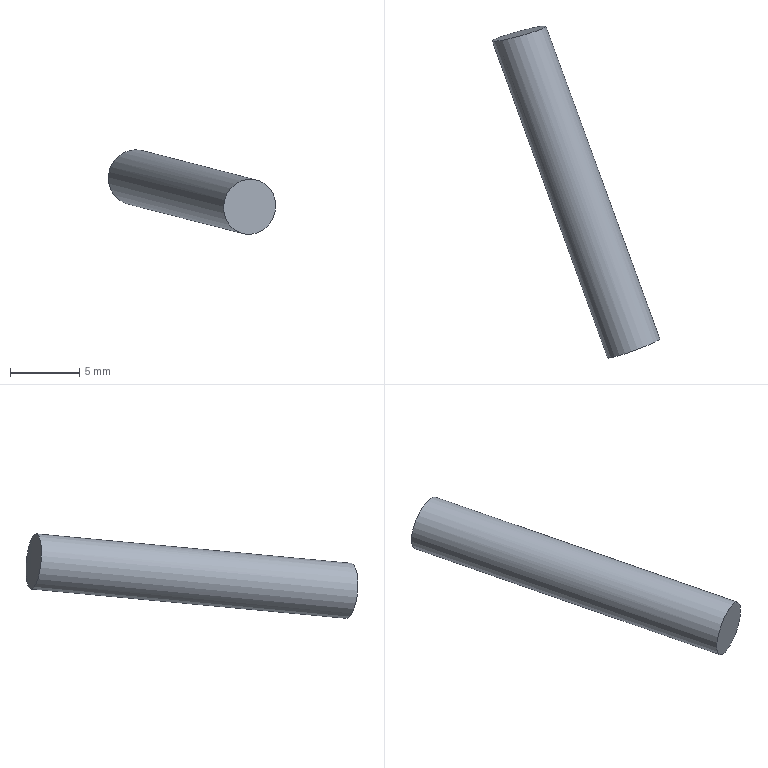Part | NX | features solid 2 | 1 solid | 3 faces | box 12.083 x 23.968 x 6.098 mm | volume 304.751 mm3 | cylinder 1 | plane 1 | spline 1 | commonest cylinder face diameters 4 x1
STEP:
#1=CARTESIAN_POINT('',(652.376,51.525,-28.692));
#2=VERTEX_POINT('',#1);
#3=CARTESIAN_POINT('',(652.847,51.506,-27.131));
#4=CARTESIAN_POINT('',(652.164,51.468,-28.691));
#5=CARTESIAN_POINT('',(652.75,51.771,-30.259));
#6=CARTESIAN_POINT('',(654.244,52.235,-30.913));
#7=CARTESIAN_POINT('',(655.778,52.598,-30.282));
#8=CARTESIAN_POINT('',(656.457,52.642,-28.723));
#9=CARTESIAN_POINT('',(655.876,52.335,-27.157));
#10=CARTESIAN_POINT('',(654.383,51.863,-26.501));
#11=CARTESIAN_POINT('',(652.847,51.506,-27.131));
#12=CARTESIAN_POINT('',(652.164,51.468,-28.691));
#13=CARTESIAN_POINT('',(652.75,51.771,-30.259));
#14=B_SPLINE_CURVE_WITH_KNOTS('',3,(#3,#4,#5,#6,#7,#8,#9,#10,#11,#12,#13),.UNSPECIFIED.,.T.,.F.,(1,1,1,1,1,1,1,1,1,1,1,1,1,1,1),(-0.004697,-0.003132,-0.001566,0.,0.001566,0.003132,0.004697,0.006263,0.007829,0.009395,0.01096,0.01253,0.01409,0.01566,0.01722),.UNSPECIFIED.);
#15=EDGE_CURVE('',#2,#2,#14,.T.);
#16=ORIENTED_EDGE('',*,*,#15,.T.);
#17=EDGE_LOOP('',(#16));
#18=FACE_BOUND('',#17,.T.);
#19=CARTESIAN_POINT('',(660.698,28.66,-30.821));
#20=VERTEX_POINT('',#19);
#21=CARTESIAN_POINT('',(662.577,29.344,-30.821));
#22=DIRECTION('',(-0.3407,0.9361,0.08716));
#23=DIRECTION('',(-0.9397,-0.342,0.));
#24=AXIS2_PLACEMENT_3D('',#21,#22,#23);
#25=CIRCLE('',#24,2.);
#26=EDGE_CURVE('',#20,#20,#25,.T.);
#27=ORIENTED_EDGE('',*,*,#26,.T.);
#28=EDGE_LOOP('',(#27));
#29=FACE_BOUND('',#28,.T.);
#30=CARTESIAN_POINT('',(654.059,52.747,-28.642));
#31=DIRECTION('',(0.3407,-0.9361,-0.08716));
#32=DIRECTION('',(-0.9397,-0.342,0.));
#33=AXIS2_PLACEMENT_3D('',#30,#31,#32);
#34=CYLINDRICAL_SURFACE('',#33,2.);
#35=ADVANCED_FACE('',(#18,#29),#34,.T.);
#36=ORIENTED_EDGE('',*,*,#26,.F.);
#37=EDGE_LOOP('',(#36));
#38=FACE_BOUND('',#37,.T.);
#39=CARTESIAN_POINT('',(662.577,29.344,-30.821));
#40=DIRECTION('',(0.3407,-0.9361,-0.08716));
#41=DIRECTION('',(-0.9397,-0.342,0.));
#42=AXIS2_PLACEMENT_3D('',#39,#40,#41);
#43=PLANE('',#42);
#44=ADVANCED_FACE('',(#38),#43,.T.);
#45=ORIENTED_EDGE('',*,*,#15,.F.);
#46=EDGE_LOOP('',(#45));
#47=FACE_BOUND('',#46,.T.);
#48=CARTESIAN_POINT('',(652.272,51.322,-26.807));
#49=CARTESIAN_POINT('',(652.413,51.736,-30.849));
#50=CARTESIAN_POINT('',(653.586,51.666,-26.726));
#51=CARTESIAN_POINT('',(653.727,52.08,-30.768));
#52=CARTESIAN_POINT('',(654.898,52.016,-26.644));
#53=CARTESIAN_POINT('',(655.039,52.43,-30.687));
#54=CARTESIAN_POINT('',(656.209,52.373,-26.562));
#55=CARTESIAN_POINT('',(656.35,52.787,-30.605));
#56=(BOUNDED_SURFACE()B_SPLINE_SURFACE(3,1,((#48,#49),(#50,#51),(#52,#53),(#54,#55)),.SURF_OF_LINEAR_EXTRUSION.,.F.,.F.,.F.)B_SPLINE_SURFACE_WITH_KNOTS((4,4),(2,2),(0.3802,0.3983),(0.4722,0.5046),.PIECEWISE_BEZIER_KNOTS.)GEOMETRIC_REPRESENTATION_ITEM()RATIONAL_B_SPLINE_SURFACE(((0.997,0.997),(0.9969,0.9969),(0.9968,0.9968),(0.9967,0.9967)))REPRESENTATION_ITEM('')SURFACE());
#57=ADVANCED_FACE('',(#47),#56,.T.);
#58=CLOSED_SHELL('',(#35,#44,#57));
#59=MANIFOLD_SOLID_BREP('',#58);
#60=(LENGTH_UNIT()NAMED_UNIT(*)SI_UNIT(.MILLI.,.METRE.));
#61=UNCERTAINTY_MEASURE_WITH_UNIT(LENGTH_MEASURE(0.0508),#60,'','');
#62=(NAMED_UNIT(*)PLANE_ANGLE_UNIT()SI_UNIT($,.RADIAN.));
#63=(NAMED_UNIT(*)SI_UNIT($,.STERADIAN.)SOLID_ANGLE_UNIT());
#64=(GEOMETRIC_REPRESENTATION_CONTEXT(3)GLOBAL_UNCERTAINTY_ASSIGNED_CONTEXT((#61))GLOBAL_UNIT_ASSIGNED_CONTEXT((#60,#62,#63))REPRESENTATION_CONTEXT('',''));
#65=ADVANCED_BREP_SHAPE_REPRESENTATION('',(#59),#64);